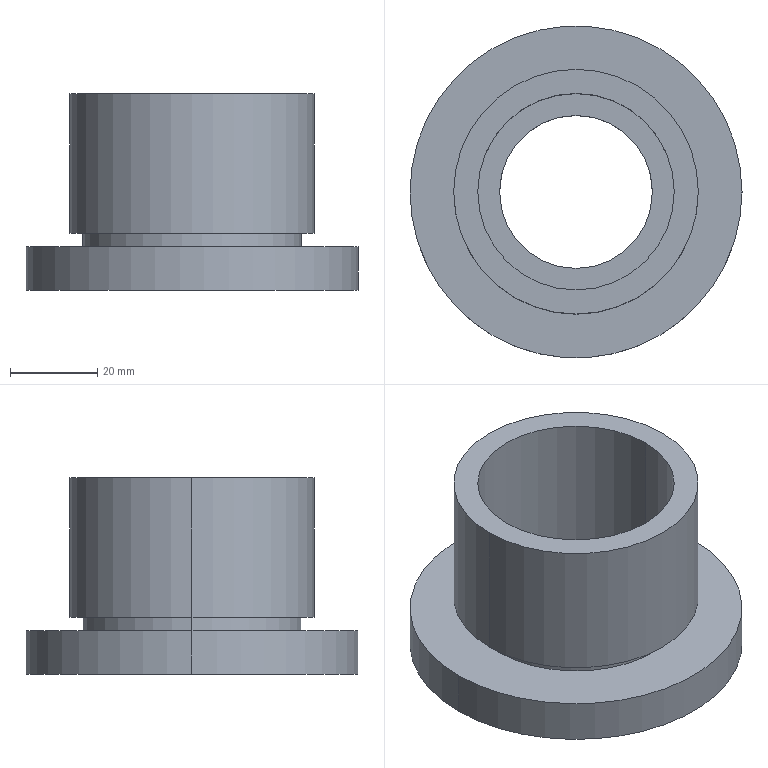Part | SolidWorks | features Revolution 1 | 1 solid | 15 faces | box 76 x 76 x 45 mm | volume 64785 mm3 | cylinder 10 | plane 5 | commonest cylinder face diameters 35 x2 45 x2 50 x2 56 x2 76 x2
STEP:
#1=CARTESIAN_POINT('',(-17.5,0.,-45.));
#2=VERTEX_POINT('',#1);
#3=CARTESIAN_POINT('',(17.5,0.,-45.));
#4=VERTEX_POINT('',#3);
#5=CARTESIAN_POINT('',(0.,0.,-45.));
#6=DIRECTION('',(0.,0.,1.));
#7=DIRECTION('',(1.,0.,0.));
#8=AXIS2_PLACEMENT_3D('',#5,#6,#7);
#9=CIRCLE('',#8,17.5);
#10=EDGE_CURVE('',#2,#4,#9,.T.);
#11=ORIENTED_EDGE('',*,*,#10,.F.);
#12=CARTESIAN_POINT('',(-17.5,0.,-35.));
#13=VERTEX_POINT('',#12);
#14=CARTESIAN_POINT('',(-17.5,0.,12.011));
#15=DIRECTION('',(0.,0.,1.));
#16=VECTOR('',#15,1000.);
#17=LINE('',#14,#16);
#18=EDGE_CURVE('',#2,#13,#17,.T.);
#19=ORIENTED_EDGE('',*,*,#18,.T.);
#20=CARTESIAN_POINT('',(17.5,0.,-35.));
#21=VERTEX_POINT('',#20);
#22=CARTESIAN_POINT('',(0.,0.,-35.));
#23=DIRECTION('',(0.,0.,1.));
#24=DIRECTION('',(1.,0.,0.));
#25=AXIS2_PLACEMENT_3D('',#22,#23,#24);
#26=CIRCLE('',#25,17.5);
#27=EDGE_CURVE('',#13,#21,#26,.T.);
#28=ORIENTED_EDGE('',*,*,#27,.T.);
#29=CARTESIAN_POINT('',(17.5,0.,12.011));
#30=DIRECTION('',(0.,0.,1.));
#31=VECTOR('',#30,1000.);
#32=LINE('',#29,#31);
#33=EDGE_CURVE('',#4,#21,#32,.T.);
#34=ORIENTED_EDGE('',*,*,#33,.F.);
#35=EDGE_LOOP('',(#11,#19,#28,#34));
#36=FACE_OUTER_BOUND('',#35,.T.);
#37=CARTESIAN_POINT('',(0.,0.,12.011));
#38=DIRECTION('',(0.,0.,1.));
#39=DIRECTION('',(1.,0.,0.));
#40=AXIS2_PLACEMENT_3D('',#37,#38,#39);
#41=CYLINDRICAL_SURFACE('',#40,17.5);
#42=ADVANCED_FACE('',(#36),#41,.F.);
#43=CARTESIAN_POINT('',(38.,0.,-45.));
#44=VERTEX_POINT('',#43);
#45=CARTESIAN_POINT('',(-38.,0.,-45.));
#46=VERTEX_POINT('',#45);
#47=CARTESIAN_POINT('',(0.,0.,-45.));
#48=DIRECTION('',(0.,0.,1.));
#49=DIRECTION('',(1.,0.,0.));
#50=AXIS2_PLACEMENT_3D('',#47,#48,#49);
#51=CIRCLE('',#50,38.);
#52=EDGE_CURVE('',#44,#46,#51,.T.);
#53=ORIENTED_EDGE('',*,*,#52,.T.);
#54=CARTESIAN_POINT('',(-38.,0.,-35.));
#55=VERTEX_POINT('',#54);
#56=CARTESIAN_POINT('',(-38.,0.,12.011));
#57=DIRECTION('',(0.,0.,1.));
#58=VECTOR('',#57,1000.);
#59=LINE('',#56,#58);
#60=EDGE_CURVE('',#46,#55,#59,.T.);
#61=ORIENTED_EDGE('',*,*,#60,.T.);
#62=CARTESIAN_POINT('',(38.,0.,-35.));
#63=VERTEX_POINT('',#62);
#64=CARTESIAN_POINT('',(0.,0.,-35.));
#65=DIRECTION('',(0.,0.,1.));
#66=DIRECTION('',(1.,0.,0.));
#67=AXIS2_PLACEMENT_3D('',#64,#65,#66);
#68=CIRCLE('',#67,38.);
#69=EDGE_CURVE('',#63,#55,#68,.T.);
#70=ORIENTED_EDGE('',*,*,#69,.F.);
#71=CARTESIAN_POINT('',(38.,0.,12.011));
#72=DIRECTION('',(0.,0.,1.));
#73=VECTOR('',#72,1000.);
#74=LINE('',#71,#73);
#75=EDGE_CURVE('',#44,#63,#74,.T.);
#76=ORIENTED_EDGE('',*,*,#75,.F.);
#77=EDGE_LOOP('',(#53,#61,#70,#76));
#78=FACE_OUTER_BOUND('',#77,.T.);
#79=CARTESIAN_POINT('',(0.,0.,12.011));
#80=DIRECTION('',(0.,0.,1.));
#81=DIRECTION('',(1.,0.,0.));
#82=AXIS2_PLACEMENT_3D('',#79,#80,#81);
#83=CYLINDRICAL_SURFACE('',#82,38.);
#84=ADVANCED_FACE('',(#78),#83,.T.);
#85=CARTESIAN_POINT('',(25.,0.,-35.));
#86=VERTEX_POINT('',#85);
#87=CARTESIAN_POINT('',(-25.,0.,-35.));
#88=VERTEX_POINT('',#87);
#89=CARTESIAN_POINT('',(0.,0.,-35.));
#90=DIRECTION('',(0.,0.,1.));
#91=DIRECTION('',(1.,0.,0.));
#92=AXIS2_PLACEMENT_3D('',#89,#90,#91);
#93=CIRCLE('',#92,25.);
#94=EDGE_CURVE('',#86,#88,#93,.T.);
#95=ORIENTED_EDGE('',*,*,#94,.T.);
#96=CARTESIAN_POINT('',(-25.,0.,-32.));
#97=VERTEX_POINT('',#96);
#98=CARTESIAN_POINT('',(-25.,0.,12.011));
#99=DIRECTION('',(0.,0.,1.));
#100=VECTOR('',#99,1000.);
#101=LINE('',#98,#100);
#102=EDGE_CURVE('',#88,#97,#101,.T.);
#103=ORIENTED_EDGE('',*,*,#102,.T.);
#104=CARTESIAN_POINT('',(25.,0.,-32.));
#105=VERTEX_POINT('',#104);
#106=CARTESIAN_POINT('',(0.,0.,-32.));
#107=DIRECTION('',(0.,0.,1.));
#108=DIRECTION('',(1.,0.,0.));
#109=AXIS2_PLACEMENT_3D('',#106,#107,#108);
#110=CIRCLE('',#109,25.);
#111=EDGE_CURVE('',#105,#97,#110,.T.);
#112=ORIENTED_EDGE('',*,*,#111,.F.);
#113=CARTESIAN_POINT('',(25.,0.,12.011));
#114=DIRECTION('',(0.,0.,1.));
#115=VECTOR('',#114,1000.);
#116=LINE('',#113,#115);
#117=EDGE_CURVE('',#86,#105,#116,.T.);
#118=ORIENTED_EDGE('',*,*,#117,.F.);
#119=EDGE_LOOP('',(#95,#103,#112,#118));
#120=FACE_OUTER_BOUND('',#119,.T.);
#121=CARTESIAN_POINT('',(0.,0.,12.011));
#122=DIRECTION('',(0.,0.,1.));
#123=DIRECTION('',(1.,0.,0.));
#124=AXIS2_PLACEMENT_3D('',#121,#122,#123);
#125=CYLINDRICAL_SURFACE('',#124,25.);
#126=ADVANCED_FACE('',(#120),#125,.T.);
#127=CARTESIAN_POINT('',(28.,0.,-32.));
#128=VERTEX_POINT('',#127);
#129=CARTESIAN_POINT('',(-28.,0.,-32.));
#130=VERTEX_POINT('',#129);
#131=CARTESIAN_POINT('',(0.,0.,-32.));
#132=DIRECTION('',(0.,0.,1.));
#133=DIRECTION('',(1.,0.,0.));
#134=AXIS2_PLACEMENT_3D('',#131,#132,#133);
#135=CIRCLE('',#134,28.);
#136=EDGE_CURVE('',#128,#130,#135,.T.);
#137=ORIENTED_EDGE('',*,*,#136,.T.);
#138=CARTESIAN_POINT('',(-28.,0.,0.));
#139=VERTEX_POINT('',#138);
#140=CARTESIAN_POINT('',(-28.,0.,12.011));
#141=DIRECTION('',(0.,0.,1.));
#142=VECTOR('',#141,1000.);
#143=LINE('',#140,#142);
#144=EDGE_CURVE('',#130,#139,#143,.T.);
#145=ORIENTED_EDGE('',*,*,#144,.T.);
#146=CARTESIAN_POINT('',(28.,0.,0.));
#147=VERTEX_POINT('',#146);
#148=CARTESIAN_POINT('',(0.,0.,0.));
#149=DIRECTION('',(0.,0.,1.));
#150=DIRECTION('',(1.,0.,0.));
#151=AXIS2_PLACEMENT_3D('',#148,#149,#150);
#152=CIRCLE('',#151,28.);
#153=EDGE_CURVE('',#147,#139,#152,.T.);
#154=ORIENTED_EDGE('',*,*,#153,.F.);
#155=CARTESIAN_POINT('',(28.,0.,12.011));
#156=DIRECTION('',(0.,0.,1.));
#157=VECTOR('',#156,1000.);
#158=LINE('',#155,#157);
#159=EDGE_CURVE('',#128,#147,#158,.T.);
#160=ORIENTED_EDGE('',*,*,#159,.F.);
#161=EDGE_LOOP('',(#137,#145,#154,#160));
#162=FACE_OUTER_BOUND('',#161,.T.);
#163=CARTESIAN_POINT('',(0.,0.,12.011));
#164=DIRECTION('',(0.,0.,1.));
#165=DIRECTION('',(1.,0.,0.));
#166=AXIS2_PLACEMENT_3D('',#163,#164,#165);
#167=CYLINDRICAL_SURFACE('',#166,28.);
#168=ADVANCED_FACE('',(#162),#167,.T.);
#169=CARTESIAN_POINT('',(-22.5,0.,-35.));
#170=VERTEX_POINT('',#169);
#171=CARTESIAN_POINT('',(22.5,0.,-35.));
#172=VERTEX_POINT('',#171);
#173=CARTESIAN_POINT('',(0.,0.,-35.));
#174=DIRECTION('',(0.,0.,1.));
#175=DIRECTION('',(1.,0.,0.));
#176=AXIS2_PLACEMENT_3D('',#173,#174,#175);
#177=CIRCLE('',#176,22.5);
#178=EDGE_CURVE('',#170,#172,#177,.T.);
#179=ORIENTED_EDGE('',*,*,#178,.F.);
#180=CARTESIAN_POINT('',(-22.5,0.,0.));
#181=VERTEX_POINT('',#180);
#182=CARTESIAN_POINT('',(-22.5,0.,12.011));
#183=DIRECTION('',(0.,0.,1.));
#184=VECTOR('',#183,1000.);
#185=LINE('',#182,#184);
#186=EDGE_CURVE('',#170,#181,#185,.T.);
#187=ORIENTED_EDGE('',*,*,#186,.T.);
#188=CARTESIAN_POINT('',(22.5,0.,0.));
#189=VERTEX_POINT('',#188);
#190=CARTESIAN_POINT('',(0.,0.,0.));
#191=DIRECTION('',(0.,0.,1.));
#192=DIRECTION('',(1.,0.,0.));
#193=AXIS2_PLACEMENT_3D('',#190,#191,#192);
#194=CIRCLE('',#193,22.5);
#195=EDGE_CURVE('',#181,#189,#194,.T.);
#196=ORIENTED_EDGE('',*,*,#195,.T.);
#197=CARTESIAN_POINT('',(22.5,0.,12.011));
#198=DIRECTION('',(0.,0.,1.));
#199=VECTOR('',#198,1000.);
#200=LINE('',#197,#199);
#201=EDGE_CURVE('',#172,#189,#200,.T.);
#202=ORIENTED_EDGE('',*,*,#201,.F.);
#203=EDGE_LOOP('',(#179,#187,#196,#202));
#204=FACE_OUTER_BOUND('',#203,.T.);
#205=CARTESIAN_POINT('',(0.,0.,12.011));
#206=DIRECTION('',(0.,0.,1.));
#207=DIRECTION('',(1.,0.,0.));
#208=AXIS2_PLACEMENT_3D('',#205,#206,#207);
#209=CYLINDRICAL_SURFACE('',#208,22.5);
#210=ADVANCED_FACE('',(#204),#209,.F.);
#211=ORIENTED_EDGE('',*,*,#186,.F.);
#212=CARTESIAN_POINT('',(0.,0.,-35.));
#213=DIRECTION('',(0.,0.,1.));
#214=DIRECTION('',(1.,0.,0.));
#215=AXIS2_PLACEMENT_3D('',#212,#213,#214);
#216=CIRCLE('',#215,22.5);
#217=EDGE_CURVE('',#172,#170,#216,.T.);
#218=ORIENTED_EDGE('',*,*,#217,.F.);
#219=ORIENTED_EDGE('',*,*,#201,.T.);
#220=CARTESIAN_POINT('',(0.,0.,0.));
#221=DIRECTION('',(0.,0.,1.));
#222=DIRECTION('',(1.,0.,0.));
#223=AXIS2_PLACEMENT_3D('',#220,#221,#222);
#224=CIRCLE('',#223,22.5);
#225=EDGE_CURVE('',#189,#181,#224,.T.);
#226=ORIENTED_EDGE('',*,*,#225,.T.);
#227=EDGE_LOOP('',(#211,#218,#219,#226));
#228=FACE_OUTER_BOUND('',#227,.T.);
#229=CARTESIAN_POINT('',(0.,0.,12.011));
#230=DIRECTION('',(0.,0.,1.));
#231=DIRECTION('',(1.,0.,0.));
#232=AXIS2_PLACEMENT_3D('',#229,#230,#231);
#233=CYLINDRICAL_SURFACE('',#232,22.5);
#234=ADVANCED_FACE('',(#228),#233,.F.);
#235=ORIENTED_EDGE('',*,*,#225,.F.);
#236=ORIENTED_EDGE('',*,*,#195,.F.);
#237=EDGE_LOOP('',(#235,#236));
#238=FACE_BOUND('',#237,.T.);
#239=ORIENTED_EDGE('',*,*,#153,.T.);
#240=CARTESIAN_POINT('',(0.,0.,0.));
#241=DIRECTION('',(0.,0.,1.));
#242=DIRECTION('',(1.,0.,0.));
#243=AXIS2_PLACEMENT_3D('',#240,#241,#242);
#244=CIRCLE('',#243,28.);
#245=EDGE_CURVE('',#139,#147,#244,.T.);
#246=ORIENTED_EDGE('',*,*,#245,.T.);
#247=EDGE_LOOP('',(#239,#246));
#248=FACE_OUTER_BOUND('',#247,.T.);
#249=CARTESIAN_POINT('',(0.,22.5,0.));
#250=DIRECTION('',(0.,0.,-1.));
#251=DIRECTION('',(-1.,0.,0.));
#252=AXIS2_PLACEMENT_3D('',#249,#250,#251);
#253=PLANE('',#252);
#254=ADVANCED_FACE('',(#238,#248),#253,.F.);
#255=ORIENTED_EDGE('',*,*,#144,.F.);
#256=CARTESIAN_POINT('',(0.,0.,-32.));
#257=DIRECTION('',(0.,0.,1.));
#258=DIRECTION('',(1.,0.,0.));
#259=AXIS2_PLACEMENT_3D('',#256,#257,#258);
#260=CIRCLE('',#259,28.);
#261=EDGE_CURVE('',#130,#128,#260,.T.);
#262=ORIENTED_EDGE('',*,*,#261,.T.);
#263=ORIENTED_EDGE('',*,*,#159,.T.);
#264=ORIENTED_EDGE('',*,*,#245,.F.);
#265=EDGE_LOOP('',(#255,#262,#263,#264));
#266=FACE_OUTER_BOUND('',#265,.T.);
#267=CARTESIAN_POINT('',(0.,0.,12.011));
#268=DIRECTION('',(0.,0.,1.));
#269=DIRECTION('',(1.,0.,0.));
#270=AXIS2_PLACEMENT_3D('',#267,#268,#269);
#271=CYLINDRICAL_SURFACE('',#270,28.);
#272=ADVANCED_FACE('',(#266),#271,.T.);
#273=ORIENTED_EDGE('',*,*,#136,.F.);
#274=ORIENTED_EDGE('',*,*,#261,.F.);
#275=EDGE_LOOP('',(#273,#274));
#276=FACE_OUTER_BOUND('',#275,.T.);
#277=ORIENTED_EDGE('',*,*,#111,.T.);
#278=CARTESIAN_POINT('',(0.,0.,-32.));
#279=DIRECTION('',(0.,0.,1.));
#280=DIRECTION('',(1.,0.,0.));
#281=AXIS2_PLACEMENT_3D('',#278,#279,#280);
#282=CIRCLE('',#281,25.);
#283=EDGE_CURVE('',#97,#105,#282,.T.);
#284=ORIENTED_EDGE('',*,*,#283,.T.);
#285=EDGE_LOOP('',(#277,#284));
#286=FACE_BOUND('',#285,.T.);
#287=CARTESIAN_POINT('',(0.,28.,-32.));
#288=DIRECTION('',(0.,0.,1.));
#289=DIRECTION('',(1.,0.,0.));
#290=AXIS2_PLACEMENT_3D('',#287,#288,#289);
#291=PLANE('',#290);
#292=ADVANCED_FACE('',(#276,#286),#291,.F.);
#293=ORIENTED_EDGE('',*,*,#102,.F.);
#294=CARTESIAN_POINT('',(0.,0.,-35.));
#295=DIRECTION('',(0.,0.,1.));
#296=DIRECTION('',(1.,0.,0.));
#297=AXIS2_PLACEMENT_3D('',#294,#295,#296);
#298=CIRCLE('',#297,25.);
#299=EDGE_CURVE('',#88,#86,#298,.T.);
#300=ORIENTED_EDGE('',*,*,#299,.T.);
#301=ORIENTED_EDGE('',*,*,#117,.T.);
#302=ORIENTED_EDGE('',*,*,#283,.F.);
#303=EDGE_LOOP('',(#293,#300,#301,#302));
#304=FACE_OUTER_BOUND('',#303,.T.);
#305=CARTESIAN_POINT('',(0.,0.,12.011));
#306=DIRECTION('',(0.,0.,1.));
#307=DIRECTION('',(1.,0.,0.));
#308=AXIS2_PLACEMENT_3D('',#305,#306,#307);
#309=CYLINDRICAL_SURFACE('',#308,25.);
#310=ADVANCED_FACE('',(#304),#309,.T.);
#311=ORIENTED_EDGE('',*,*,#94,.F.);
#312=ORIENTED_EDGE('',*,*,#299,.F.);
#313=EDGE_LOOP('',(#311,#312));
#314=FACE_BOUND('',#313,.T.);
#315=ORIENTED_EDGE('',*,*,#69,.T.);
#316=CARTESIAN_POINT('',(0.,0.,-35.));
#317=DIRECTION('',(0.,0.,1.));
#318=DIRECTION('',(1.,0.,0.));
#319=AXIS2_PLACEMENT_3D('',#316,#317,#318);
#320=CIRCLE('',#319,38.);
#321=EDGE_CURVE('',#55,#63,#320,.T.);
#322=ORIENTED_EDGE('',*,*,#321,.T.);
#323=EDGE_LOOP('',(#315,#322));
#324=FACE_OUTER_BOUND('',#323,.T.);
#325=CARTESIAN_POINT('',(0.,25.,-35.));
#326=DIRECTION('',(0.,0.,-1.));
#327=DIRECTION('',(-1.,0.,0.));
#328=AXIS2_PLACEMENT_3D('',#325,#326,#327);
#329=PLANE('',#328);
#330=ADVANCED_FACE('',(#314,#324),#329,.F.);
#331=ORIENTED_EDGE('',*,*,#60,.F.);
#332=CARTESIAN_POINT('',(0.,0.,-45.));
#333=DIRECTION('',(0.,0.,1.));
#334=DIRECTION('',(1.,0.,0.));
#335=AXIS2_PLACEMENT_3D('',#332,#333,#334);
#336=CIRCLE('',#335,38.);
#337=EDGE_CURVE('',#46,#44,#336,.T.);
#338=ORIENTED_EDGE('',*,*,#337,.T.);
#339=ORIENTED_EDGE('',*,*,#75,.T.);
#340=ORIENTED_EDGE('',*,*,#321,.F.);
#341=EDGE_LOOP('',(#331,#338,#339,#340));
#342=FACE_OUTER_BOUND('',#341,.T.);
#343=CARTESIAN_POINT('',(0.,0.,12.011));
#344=DIRECTION('',(0.,0.,1.));
#345=DIRECTION('',(1.,0.,0.));
#346=AXIS2_PLACEMENT_3D('',#343,#344,#345);
#347=CYLINDRICAL_SURFACE('',#346,38.);
#348=ADVANCED_FACE('',(#342),#347,.T.);
#349=ORIENTED_EDGE('',*,*,#52,.F.);
#350=ORIENTED_EDGE('',*,*,#337,.F.);
#351=EDGE_LOOP('',(#349,#350));
#352=FACE_OUTER_BOUND('',#351,.T.);
#353=CARTESIAN_POINT('',(0.,0.,-45.));
#354=DIRECTION('',(0.,0.,1.));
#355=DIRECTION('',(1.,0.,0.));
#356=AXIS2_PLACEMENT_3D('',#353,#354,#355);
#357=CIRCLE('',#356,17.5);
#358=EDGE_CURVE('',#4,#2,#357,.T.);
#359=ORIENTED_EDGE('',*,*,#358,.T.);
#360=ORIENTED_EDGE('',*,*,#10,.T.);
#361=EDGE_LOOP('',(#359,#360));
#362=FACE_BOUND('',#361,.T.);
#363=CARTESIAN_POINT('',(0.,38.,-45.));
#364=DIRECTION('',(0.,0.,1.));
#365=DIRECTION('',(1.,0.,0.));
#366=AXIS2_PLACEMENT_3D('',#363,#364,#365);
#367=PLANE('',#366);
#368=ADVANCED_FACE('',(#352,#362),#367,.F.);
#369=ORIENTED_EDGE('',*,*,#18,.F.);
#370=ORIENTED_EDGE('',*,*,#358,.F.);
#371=ORIENTED_EDGE('',*,*,#33,.T.);
#372=CARTESIAN_POINT('',(0.,0.,-35.));
#373=DIRECTION('',(0.,0.,1.));
#374=DIRECTION('',(1.,0.,0.));
#375=AXIS2_PLACEMENT_3D('',#372,#373,#374);
#376=CIRCLE('',#375,17.5);
#377=EDGE_CURVE('',#21,#13,#376,.T.);
#378=ORIENTED_EDGE('',*,*,#377,.T.);
#379=EDGE_LOOP('',(#369,#370,#371,#378));
#380=FACE_OUTER_BOUND('',#379,.T.);
#381=CARTESIAN_POINT('',(0.,0.,12.011));
#382=DIRECTION('',(0.,0.,1.));
#383=DIRECTION('',(1.,0.,0.));
#384=AXIS2_PLACEMENT_3D('',#381,#382,#383);
#385=CYLINDRICAL_SURFACE('',#384,17.5);
#386=ADVANCED_FACE('',(#380),#385,.F.);
#387=ORIENTED_EDGE('',*,*,#377,.F.);
#388=ORIENTED_EDGE('',*,*,#27,.F.);
#389=EDGE_LOOP('',(#387,#388));
#390=FACE_BOUND('',#389,.T.);
#391=ORIENTED_EDGE('',*,*,#217,.T.);
#392=ORIENTED_EDGE('',*,*,#178,.T.);
#393=EDGE_LOOP('',(#391,#392));
#394=FACE_OUTER_BOUND('',#393,.T.);
#395=CARTESIAN_POINT('',(0.,17.5,-35.));
#396=DIRECTION('',(0.,0.,-1.));
#397=DIRECTION('',(-1.,0.,0.));
#398=AXIS2_PLACEMENT_3D('',#395,#396,#397);
#399=PLANE('',#398);
#400=ADVANCED_FACE('',(#390,#394),#399,.F.);
#401=CLOSED_SHELL('',(#42,#84,#126,#168,#210,#234,#254,#272,#292,#310,#330,#348,#368,#386,#400));
#402=MANIFOLD_SOLID_BREP('',#401);
#403=CARTESIAN_POINT('',(0.,0.,0.));
#404=DIRECTION('',(0.,0.,1.));
#405=DIRECTION('',(1.,0.,0.));
#406=AXIS2_PLACEMENT_3D('',#403,#404,#405);
#407=(LENGTH_UNIT()NAMED_UNIT(*)SI_UNIT(.MILLI.,.METRE.));
#408=UNCERTAINTY_MEASURE_WITH_UNIT(LENGTH_MEASURE(0.00001),#407,'','');
#409=(NAMED_UNIT(*)PLANE_ANGLE_UNIT()SI_UNIT($,.RADIAN.));
#410=(NAMED_UNIT(*)SI_UNIT($,.STERADIAN.)SOLID_ANGLE_UNIT());
#411=(GEOMETRIC_REPRESENTATION_CONTEXT(3)GLOBAL_UNCERTAINTY_ASSIGNED_CONTEXT((#408))GLOBAL_UNIT_ASSIGNED_CONTEXT((#407,#409,#410))REPRESENTATION_CONTEXT('',''));
#412=ADVANCED_BREP_SHAPE_REPRESENTATION('',(#402,#406),#411);